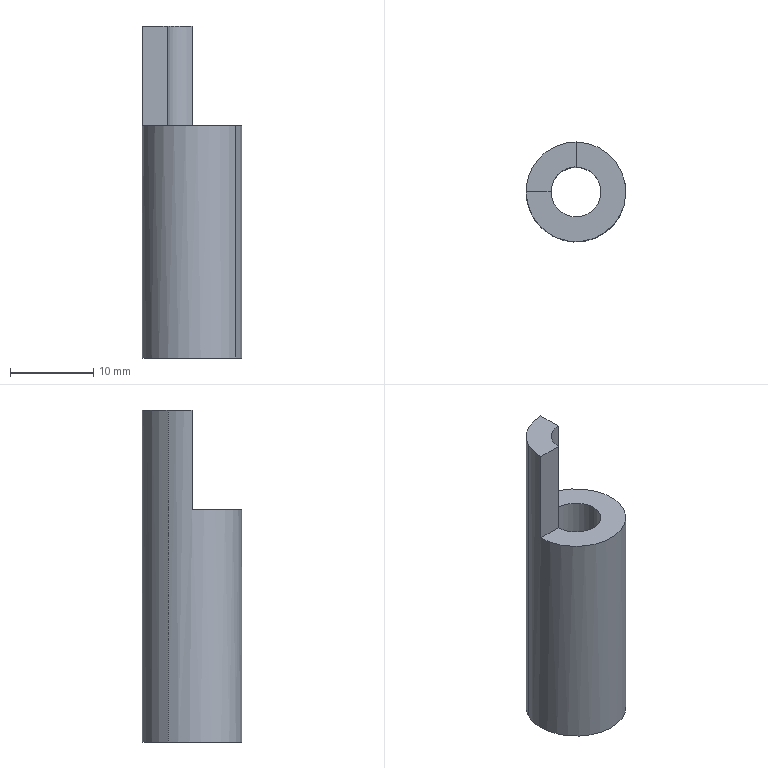Part | CATIA | 1 solid | 9 faces | box 12 x 12 x 40 mm | volume 2630 mm3 | plane 5 | cylinder 4 | commonest cylinder face diameters 6 x2 12 x2
STEP:
#1=CARTESIAN_POINT('',(5.265,-2.877,-28.));
#2=VERTEX_POINT('',#1);
#3=CARTESIAN_POINT('',(-5.265,2.877,-28.));
#4=VERTEX_POINT('',#3);
#5=CARTESIAN_POINT('',(0.,0.,-28.));
#6=DIRECTION('',(0.,0.,1.));
#7=AXIS2_PLACEMENT_3D('',#5,#6,$);
#8=CIRCLE('',#7,6.);
#9=EDGE_CURVE('',#2,#4,#8,.T.);
#10=ORIENTED_EDGE('',*,*,#9,.F.);
#11=CARTESIAN_POINT('',(0.,0.,-28.));
#12=DIRECTION('',(0.,0.,1.));
#13=AXIS2_PLACEMENT_3D('',#11,#12,$);
#14=CIRCLE('',#13,6.);
#15=EDGE_CURVE('',#4,#2,#14,.T.);
#16=ORIENTED_EDGE('',*,*,#15,.F.);
#17=EDGE_LOOP('',(#10,#16));
#18=FACE_OUTER_BOUND('',#17,.T.);
#19=CARTESIAN_POINT('',(3.,0.,-28.));
#20=VERTEX_POINT('',#19);
#21=CARTESIAN_POINT('',(-3.,0.,-28.));
#22=VERTEX_POINT('',#21);
#23=CARTESIAN_POINT('',(0.,0.,-28.));
#24=DIRECTION('',(0.,0.,1.));
#25=AXIS2_PLACEMENT_3D('',#23,#24,$);
#26=CIRCLE('',#25,3.);
#27=EDGE_CURVE('',#20,#22,#26,.T.);
#28=ORIENTED_EDGE('',*,*,#27,.T.);
#29=CARTESIAN_POINT('',(0.,0.,-28.));
#30=DIRECTION('',(0.,0.,1.));
#31=AXIS2_PLACEMENT_3D('',#29,#30,$);
#32=CIRCLE('',#31,3.);
#33=EDGE_CURVE('',#22,#20,#32,.T.);
#34=ORIENTED_EDGE('',*,*,#33,.T.);
#35=EDGE_LOOP('',(#28,#34));
#36=FACE_BOUND('',#35,.T.);
#37=CARTESIAN_POINT('',(0.,0.,-28.));
#38=DIRECTION('',(0.,0.,1.));
#39=DIRECTION('',(1.,0.,0.));
#40=AXIS2_PLACEMENT_3D('',#37,#38,#39);
#41=PLANE('',#40);
#42=ADVANCED_FACE('',(#18,#36),#41,.F.);
#43=CARTESIAN_POINT('',(0.,6.,12.));
#44=VERTEX_POINT('',#43);
#45=CARTESIAN_POINT('',(-5.265,2.877,12.));
#46=VERTEX_POINT('',#45);
#47=CARTESIAN_POINT('',(0.,0.,12.));
#48=DIRECTION('',(0.,0.,1.));
#49=AXIS2_PLACEMENT_3D('',#47,#48,$);
#50=CIRCLE('',#49,6.);
#51=EDGE_CURVE('',#44,#46,#50,.T.);
#52=ORIENTED_EDGE('',*,*,#51,.T.);
#53=CARTESIAN_POINT('',(-6.,0.,12.));
#54=VERTEX_POINT('',#53);
#55=CARTESIAN_POINT('',(0.,0.,12.));
#56=DIRECTION('',(0.,0.,1.));
#57=AXIS2_PLACEMENT_3D('',#55,#56,$);
#58=CIRCLE('',#57,6.);
#59=EDGE_CURVE('',#46,#54,#58,.T.);
#60=ORIENTED_EDGE('',*,*,#59,.T.);
#61=CARTESIAN_POINT('',(-3.,0.,12.));
#62=VERTEX_POINT('',#61);
#63=CARTESIAN_POINT('',(-4.5,0.,12.));
#64=DIRECTION('',(1.,0.,0.));
#65=VECTOR('',#64,1.);
#66=LINE('',#63,#65);
#67=EDGE_CURVE('',#62,#54,#66,.F.);
#68=ORIENTED_EDGE('',*,*,#67,.F.);
#69=CARTESIAN_POINT('',(0.,3.,12.));
#70=VERTEX_POINT('',#69);
#71=CARTESIAN_POINT('',(0.,0.,12.));
#72=DIRECTION('',(0.,0.,1.));
#73=AXIS2_PLACEMENT_3D('',#71,#72,$);
#74=CIRCLE('',#73,3.);
#75=EDGE_CURVE('',#70,#62,#74,.T.);
#76=ORIENTED_EDGE('',*,*,#75,.F.);
#77=CARTESIAN_POINT('',(0.,4.5,12.));
#78=DIRECTION('',(0.,1.,0.));
#79=VECTOR('',#78,1.);
#80=LINE('',#77,#79);
#81=EDGE_CURVE('',#44,#70,#80,.F.);
#82=ORIENTED_EDGE('',*,*,#81,.F.);
#83=EDGE_LOOP('',(#52,#60,#68,#76,#82));
#84=FACE_OUTER_BOUND('',#83,.T.);
#85=CARTESIAN_POINT('',(0.,0.,12.));
#86=DIRECTION('',(0.,0.,1.));
#87=DIRECTION('',(1.,0.,0.));
#88=AXIS2_PLACEMENT_3D('',#85,#86,#87);
#89=PLANE('',#88);
#90=ADVANCED_FACE('',(#84),#89,.T.);
#91=CARTESIAN_POINT('',(3.,0.,0.));
#92=VERTEX_POINT('',#91);
#93=CARTESIAN_POINT('',(0.,3.,0.));
#94=VERTEX_POINT('',#93);
#95=CARTESIAN_POINT('',(0.,0.,0.));
#96=DIRECTION('',(0.,0.,1.));
#97=AXIS2_PLACEMENT_3D('',#95,#96,$);
#98=CIRCLE('',#97,3.);
#99=EDGE_CURVE('',#92,#94,#98,.T.);
#100=ORIENTED_EDGE('',*,*,#99,.T.);
#101=CARTESIAN_POINT('',(0.,3.,-8.));
#102=DIRECTION('',(0.,0.,1.));
#103=VECTOR('',#102,1.);
#104=LINE('',#101,#103);
#105=EDGE_CURVE('',#70,#94,#104,.F.);
#106=ORIENTED_EDGE('',*,*,#105,.F.);
#107=ORIENTED_EDGE('',*,*,#75,.T.);
#108=CARTESIAN_POINT('',(-3.,0.,0.));
#109=VERTEX_POINT('',#108);
#110=CARTESIAN_POINT('',(-3.,0.,-8.));
#111=DIRECTION('',(0.,0.,1.));
#112=VECTOR('',#111,1.);
#113=LINE('',#110,#112);
#114=EDGE_CURVE('',#62,#109,#113,.F.);
#115=ORIENTED_EDGE('',*,*,#114,.T.);
#116=CARTESIAN_POINT('',(-3.,0.,-8.));
#117=DIRECTION('',(0.,0.,1.));
#118=VECTOR('',#117,1.);
#119=LINE('',#116,#118);
#120=EDGE_CURVE('',#109,#22,#119,.F.);
#121=ORIENTED_EDGE('',*,*,#120,.T.);
#122=ORIENTED_EDGE('',*,*,#27,.F.);
#123=CARTESIAN_POINT('',(3.,0.,-8.));
#124=DIRECTION('',(0.,0.,1.));
#125=VECTOR('',#124,1.);
#126=LINE('',#123,#125);
#127=EDGE_CURVE('',#92,#20,#126,.F.);
#128=ORIENTED_EDGE('',*,*,#127,.F.);
#129=EDGE_LOOP('',(#100,#106,#107,#115,#121,#122,#128));
#130=FACE_OUTER_BOUND('',#129,.T.);
#131=CARTESIAN_POINT('',(0.,0.,-8.));
#132=DIRECTION('',(0.,0.,1.));
#133=DIRECTION('',(1.,0.,0.));
#134=AXIS2_PLACEMENT_3D('',#131,#132,#133);
#135=CYLINDRICAL_SURFACE('',#134,3.);
#136=ADVANCED_FACE('',(#130),#135,.F.);
#137=CARTESIAN_POINT('',(0.,0.,0.));
#138=DIRECTION('',(0.,0.,1.));
#139=AXIS2_PLACEMENT_3D('',#137,#138,$);
#140=CIRCLE('',#139,3.);
#141=EDGE_CURVE('',#109,#92,#140,.T.);
#142=ORIENTED_EDGE('',*,*,#141,.T.);
#143=ORIENTED_EDGE('',*,*,#127,.T.);
#144=ORIENTED_EDGE('',*,*,#33,.F.);
#145=ORIENTED_EDGE('',*,*,#120,.F.);
#146=EDGE_LOOP('',(#142,#143,#144,#145));
#147=FACE_OUTER_BOUND('',#146,.T.);
#148=ADVANCED_FACE('',(#147),#135,.F.);
#149=CARTESIAN_POINT('',(5.265,-2.877,0.));
#150=VERTEX_POINT('',#149);
#151=CARTESIAN_POINT('',(5.265,-2.877,-8.));
#152=DIRECTION('',(0.,0.,1.));
#153=VECTOR('',#152,1.);
#154=LINE('',#151,#153);
#155=EDGE_CURVE('',#150,#2,#154,.F.);
#156=ORIENTED_EDGE('',*,*,#155,.T.);
#157=ORIENTED_EDGE('',*,*,#9,.T.);
#158=CARTESIAN_POINT('',(-5.265,2.877,-8.));
#159=DIRECTION('',(0.,0.,1.));
#160=VECTOR('',#159,1.);
#161=LINE('',#158,#160);
#162=EDGE_CURVE('',#46,#4,#161,.F.);
#163=ORIENTED_EDGE('',*,*,#162,.F.);
#164=ORIENTED_EDGE('',*,*,#51,.F.);
#165=CARTESIAN_POINT('',(0.,6.,0.));
#166=VERTEX_POINT('',#165);
#167=CARTESIAN_POINT('',(0.,6.,-8.));
#168=DIRECTION('',(0.,0.,1.));
#169=VECTOR('',#168,1.);
#170=LINE('',#167,#169);
#171=EDGE_CURVE('',#44,#166,#170,.F.);
#172=ORIENTED_EDGE('',*,*,#171,.T.);
#173=CARTESIAN_POINT('',(0.,0.,0.));
#174=DIRECTION('',(0.,0.,1.));
#175=AXIS2_PLACEMENT_3D('',#173,#174,$);
#176=CIRCLE('',#175,6.);
#177=EDGE_CURVE('',#150,#166,#176,.T.);
#178=ORIENTED_EDGE('',*,*,#177,.F.);
#179=EDGE_LOOP('',(#156,#157,#163,#164,#172,#178));
#180=FACE_OUTER_BOUND('',#179,.T.);
#181=CARTESIAN_POINT('',(0.,0.,-8.));
#182=DIRECTION('',(0.,0.,1.));
#183=DIRECTION('',(-0.8776,0.4794,0.));
#184=AXIS2_PLACEMENT_3D('',#181,#182,#183);
#185=CYLINDRICAL_SURFACE('',#184,6.);
#186=ADVANCED_FACE('',(#180),#185,.T.);
#187=ORIENTED_EDGE('',*,*,#59,.F.);
#188=ORIENTED_EDGE('',*,*,#162,.T.);
#189=ORIENTED_EDGE('',*,*,#15,.T.);
#190=ORIENTED_EDGE('',*,*,#155,.F.);
#191=CARTESIAN_POINT('',(-6.,0.,0.));
#192=VERTEX_POINT('',#191);
#193=CARTESIAN_POINT('',(0.,0.,0.));
#194=DIRECTION('',(0.,0.,1.));
#195=AXIS2_PLACEMENT_3D('',#193,#194,$);
#196=CIRCLE('',#195,6.);
#197=EDGE_CURVE('',#192,#150,#196,.T.);
#198=ORIENTED_EDGE('',*,*,#197,.F.);
#199=CARTESIAN_POINT('',(-6.,0.,-8.));
#200=DIRECTION('',(0.,0.,1.));
#201=VECTOR('',#200,1.);
#202=LINE('',#199,#201);
#203=EDGE_CURVE('',#54,#192,#202,.F.);
#204=ORIENTED_EDGE('',*,*,#203,.F.);
#205=EDGE_LOOP('',(#187,#188,#189,#190,#198,#204));
#206=FACE_OUTER_BOUND('',#205,.T.);
#207=ADVANCED_FACE('',(#206),#185,.T.);
#208=ORIENTED_EDGE('',*,*,#197,.T.);
#209=ORIENTED_EDGE('',*,*,#177,.T.);
#210=CARTESIAN_POINT('',(0.,4.5,0.));
#211=DIRECTION('',(0.,1.,0.));
#212=VECTOR('',#211,1.);
#213=LINE('',#210,#212);
#214=EDGE_CURVE('',#166,#94,#213,.F.);
#215=ORIENTED_EDGE('',*,*,#214,.T.);
#216=ORIENTED_EDGE('',*,*,#99,.F.);
#217=ORIENTED_EDGE('',*,*,#141,.F.);
#218=CARTESIAN_POINT('',(-4.5,0.,0.));
#219=DIRECTION('',(1.,0.,0.));
#220=VECTOR('',#219,1.);
#221=LINE('',#218,#220);
#222=EDGE_CURVE('',#109,#192,#221,.F.);
#223=ORIENTED_EDGE('',*,*,#222,.T.);
#224=EDGE_LOOP('',(#208,#209,#215,#216,#217,#223));
#225=FACE_OUTER_BOUND('',#224,.T.);
#226=CARTESIAN_POINT('',(0.,0.,0.));
#227=DIRECTION('',(0.,0.,1.));
#228=DIRECTION('',(1.,0.,0.));
#229=AXIS2_PLACEMENT_3D('',#226,#227,#228);
#230=PLANE('',#229);
#231=ADVANCED_FACE('',(#225),#230,.T.);
#232=ORIENTED_EDGE('',*,*,#214,.F.);
#233=ORIENTED_EDGE('',*,*,#171,.F.);
#234=ORIENTED_EDGE('',*,*,#81,.T.);
#235=ORIENTED_EDGE('',*,*,#105,.T.);
#236=EDGE_LOOP('',(#232,#233,#234,#235));
#237=FACE_OUTER_BOUND('',#236,.T.);
#238=CARTESIAN_POINT('',(0.,0.,12.));
#239=DIRECTION('',(-1.,0.,0.));
#240=DIRECTION('',(0.,1.,0.));
#241=AXIS2_PLACEMENT_3D('',#238,#239,#240);
#242=PLANE('',#241);
#243=ADVANCED_FACE('',(#237),#242,.F.);
#244=ORIENTED_EDGE('',*,*,#222,.F.);
#245=ORIENTED_EDGE('',*,*,#114,.F.);
#246=ORIENTED_EDGE('',*,*,#67,.T.);
#247=ORIENTED_EDGE('',*,*,#203,.T.);
#248=EDGE_LOOP('',(#244,#245,#246,#247));
#249=FACE_OUTER_BOUND('',#248,.T.);
#250=CARTESIAN_POINT('',(-15.,0.,12.));
#251=DIRECTION('',(0.,1.,0.));
#252=DIRECTION('',(1.,0.,0.));
#253=AXIS2_PLACEMENT_3D('',#250,#251,#252);
#254=PLANE('',#253);
#255=ADVANCED_FACE('',(#249),#254,.F.);
#256=CLOSED_SHELL('',(#42,#90,#136,#148,#186,#207,#231,#243,#255));
#257=MANIFOLD_SOLID_BREP('',#256);
#258=(LENGTH_UNIT()NAMED_UNIT(*)SI_UNIT(.MILLI.,.METRE.));
#259=UNCERTAINTY_MEASURE_WITH_UNIT(LENGTH_MEASURE(0.005),#258,'','');
#260=(NAMED_UNIT(*)PLANE_ANGLE_UNIT()SI_UNIT($,.RADIAN.));
#261=(NAMED_UNIT(*)SI_UNIT($,.STERADIAN.)SOLID_ANGLE_UNIT());
#262=(GEOMETRIC_REPRESENTATION_CONTEXT(3)GLOBAL_UNCERTAINTY_ASSIGNED_CONTEXT((#259))GLOBAL_UNIT_ASSIGNED_CONTEXT((#258,#260,#261))REPRESENTATION_CONTEXT('',''));
#263=ADVANCED_BREP_SHAPE_REPRESENTATION('',(#257),#262);